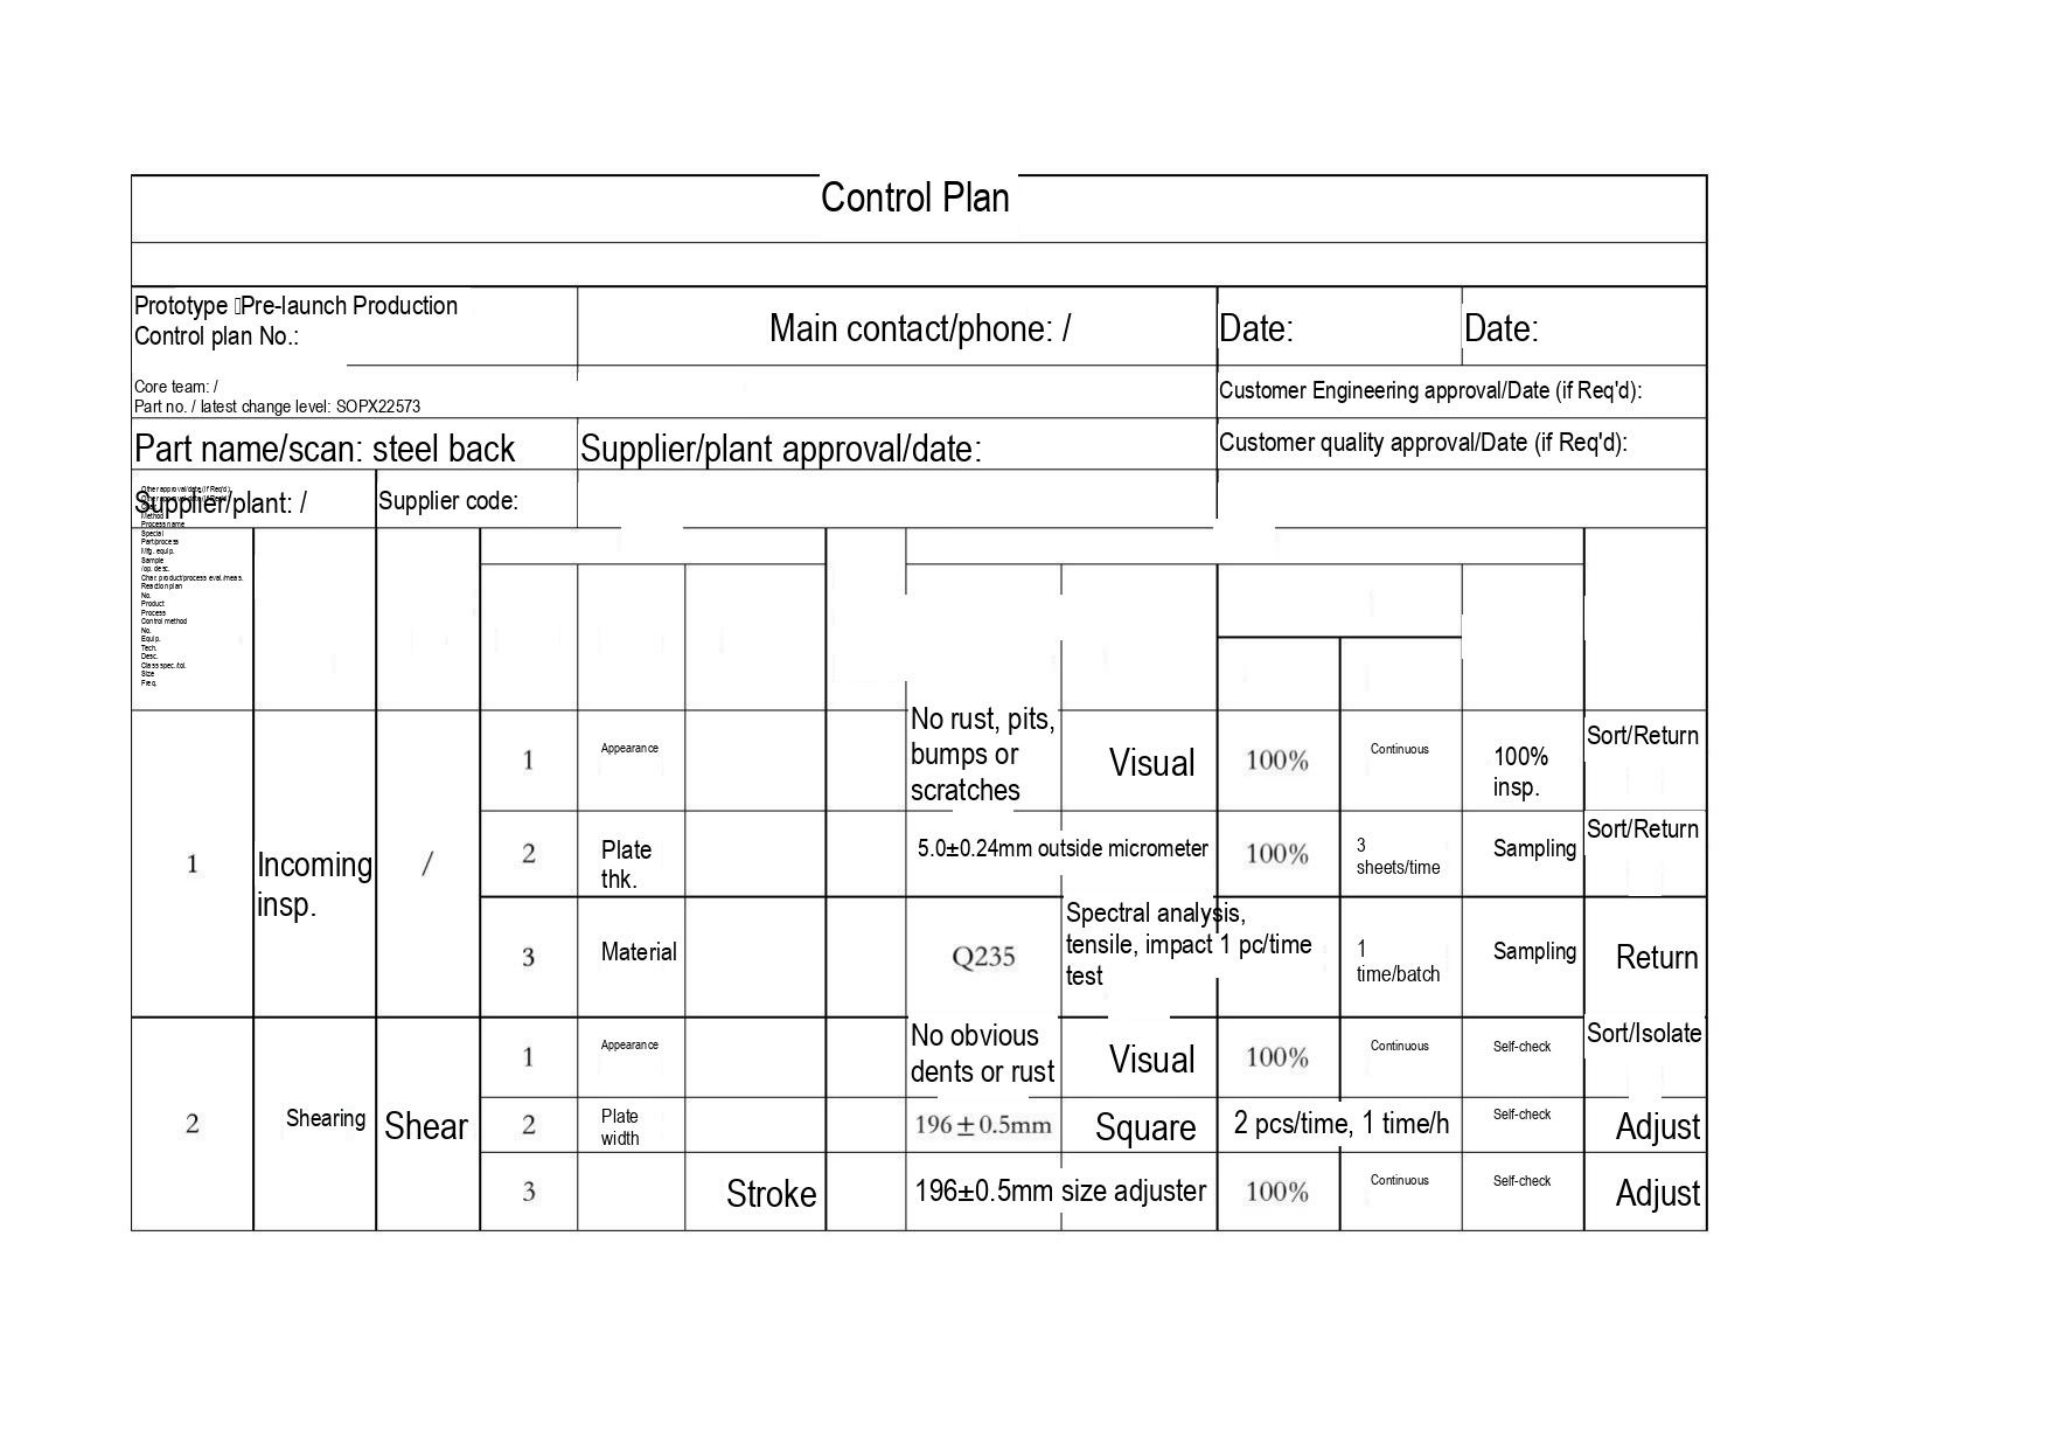Control Plan

| | | | |
|---|---|---|---|
| Prototype Pre-launch Production<br>Control plan No.: | Main contact/phone: / | Date: | Date: |
| Core team: /<br>Part no. / latest change level: SOPX22573 | | Customer Engineering approval/Date (if Req'd): | |
| Part name/scan: steel back | Supplier/plant approval/date: | Customer quality approval/Date (if Req'd): | |
| Supplier/plant: / | Supplier code: | | |

Other approval/date (If Req'd)
Method
Process name
Special
Part/process
Mfg. equip.
Sample
Op. desc.
Char. product/process eval./meas.
Reaction plan
No.
Product
Process
Control method
No.
Equip.
Tech.
Desc.
Class spec./tol.
Size
Freq.

| | | | | | | | | | | | | |
|---|---|---|---|---|---|---|---|---|---|---|---|---|
| 1 | Incoming insp. | / | 1 | Appearance | | | No rust, pits, bumps or scratches | Visual | 100% | Continuous | 100% insp. | Sort/Return |
| | | | 2 | Plate thk. | | | 5.0±0.24mm | outside micrometer | 100% | 3 sheets/time | Sampling | Sort/Return |
| | | | 3 | Material | | | Q235 | Spectral analysis, tensile, impact test | 1 pc/time | 1 time/batch | Sampling | Return |
| 2 | Shearing | Shear | 1 | Appearance | | | No obvious dents or rust | Visual | 100% | Continuous | Self-check | Sort/Isolate |
| | | | 2 | Plate width | | | 196±0.5mm | Square | 2 pcs/time, 1 time/h | | Self-check | Adjust |
| | | | 3 | | Stroke | | 196±0.5mm | size adjuster | 100% | Continuous | Self-check | Adjust |
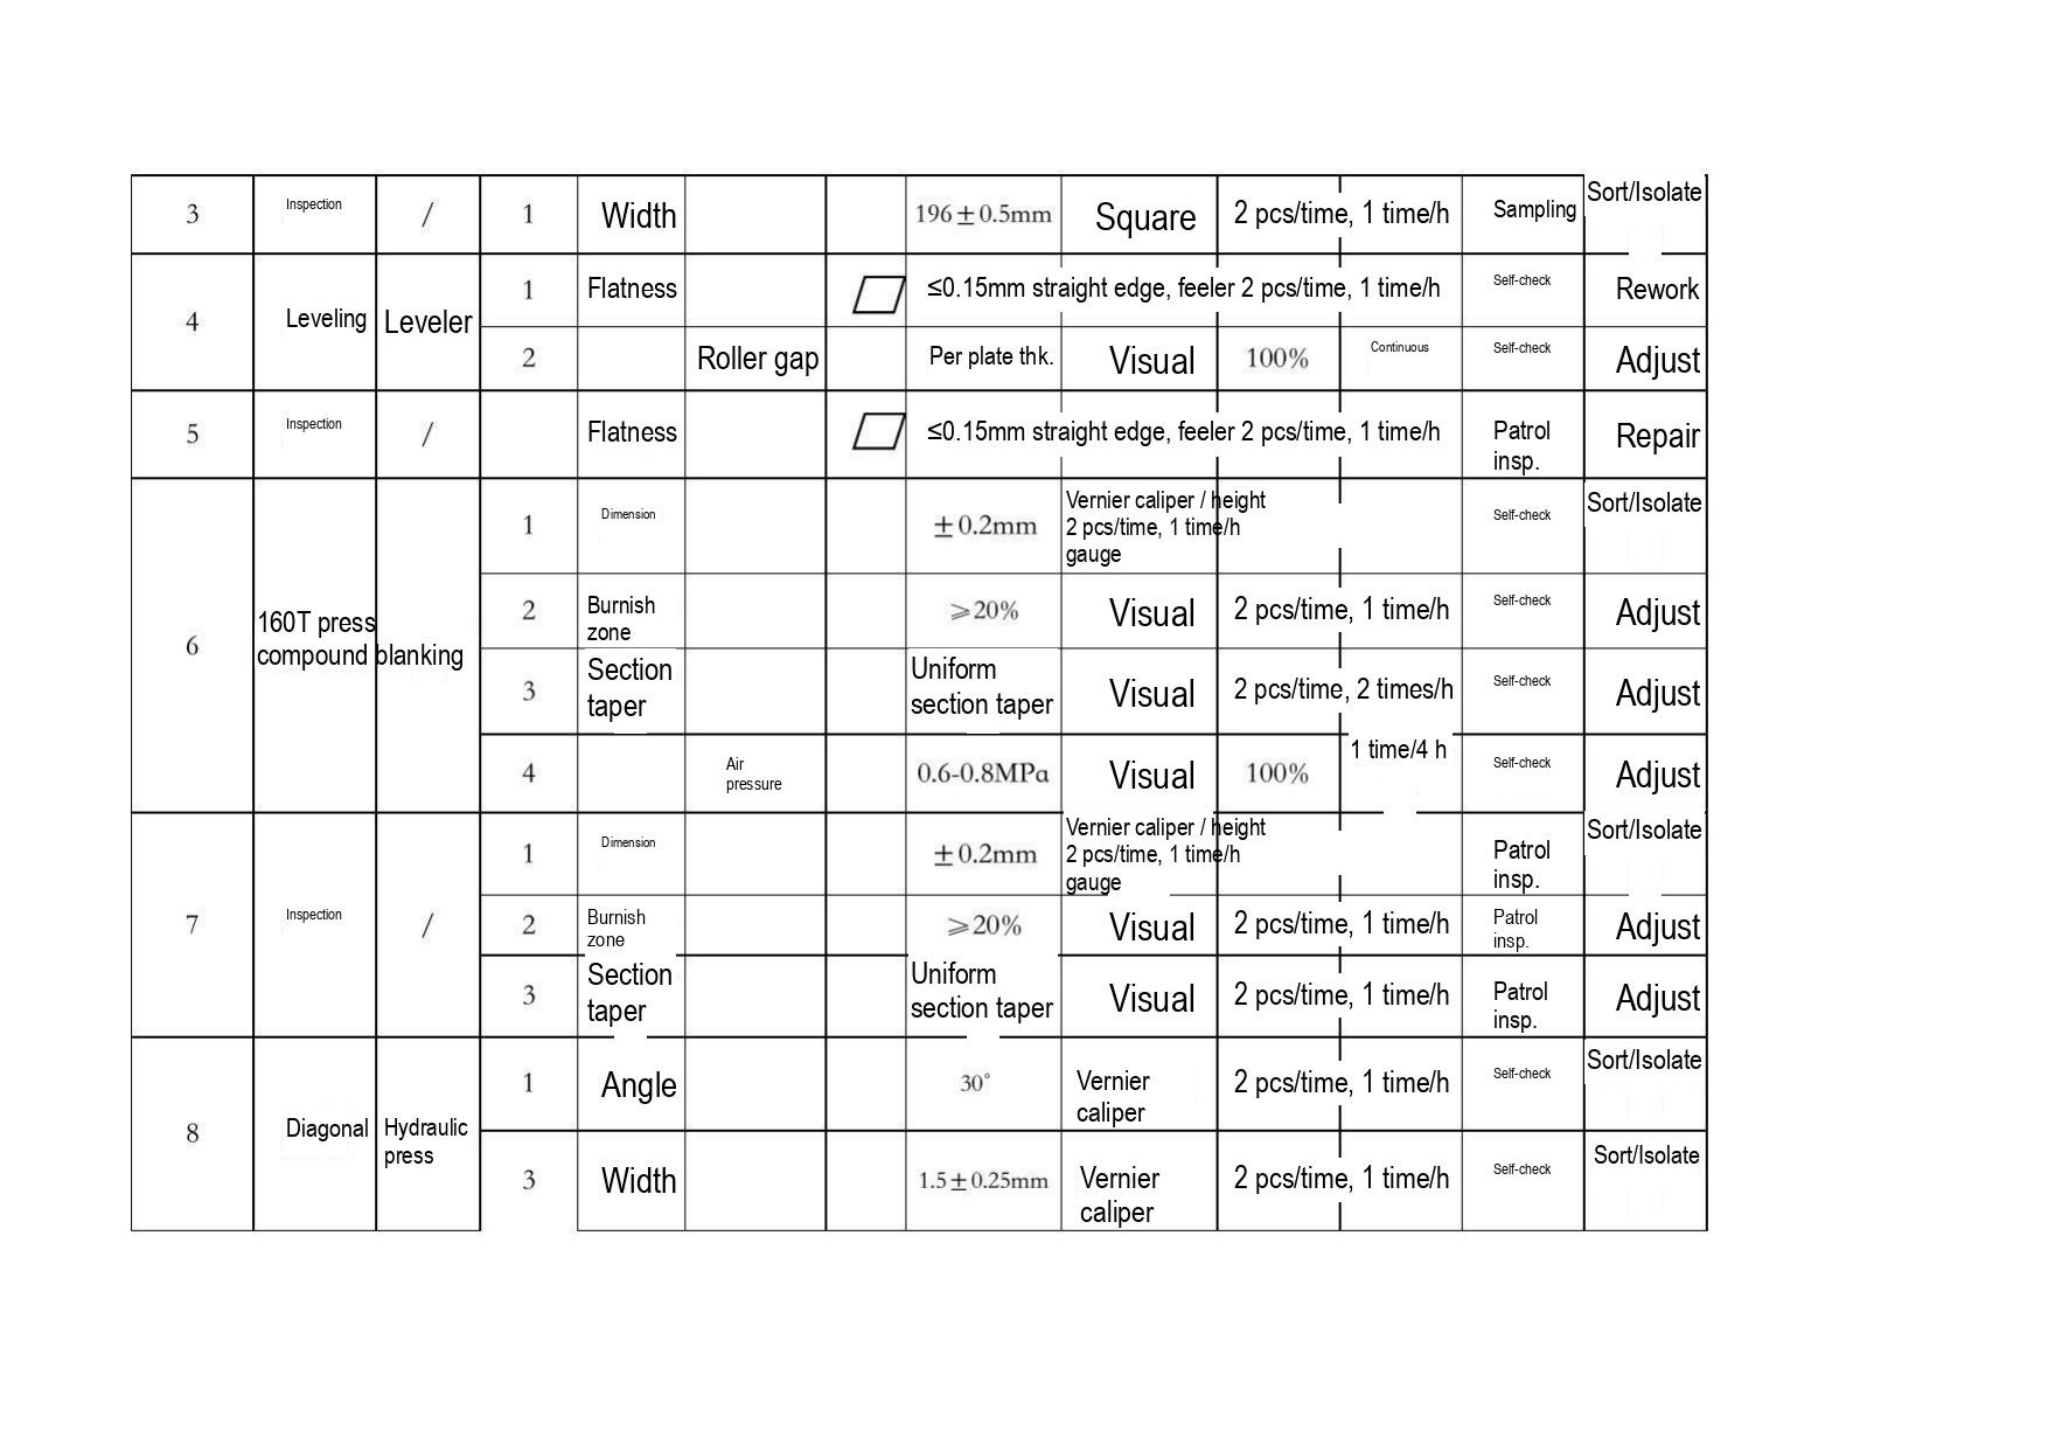|  |  |  |  |  |  |  |  |  |  |  |  |  |
|---|---|---|---|---|---|---|---|---|---|---|---|---|
| 3 | Inspection | / | 1 | Width |  |  | 196±0.5mm | Square | 2 pcs/time, 1 time/h |  | Sampling | Sort/Isolate |
| 4 | Leveling | Leveler | 1 | Flatness |  | ▱ | ≤0.15mm | straight edge, feeler | 2 pcs/time, 1 time/h |  | Self-check | Rework |
|  |  |  | 2 |  | Roller gap |  | Per plate thk. | Visual | 100% | Continuous | Self-check | Adjust |
| 5 | Inspection | / |  | Flatness |  | ▱ | ≤0.15mm | straight edge, feeler | 2 pcs/time, 1 time/h |  | Patrol insp. | Repair |
| 6 | 160T press compound blanking |  | 1 | Dimension |  |  | ±0.2mm | Vernier caliper / height gauge | 2 pcs/time, 1 time/h |  | Self-check | Sort/Isolate |
|  |  |  | 2 | Burnish zone |  |  | ≥20% | Visual | 2 pcs/time, 1 time/h |  | Self-check | Adjust |
|  |  |  | 3 | Section taper |  |  | Uniform section taper | Visual | 2 pcs/time, 2 times/h |  | Self-check | Adjust |
|  |  |  | 4 |  | Air pressure |  | 0.6-0.8MPa | Visual | 100% | 1 time/4 h | Self-check | Adjust |
| 7 | Inspection | / | 1 | Dimension |  |  | ±0.2mm | Vernier caliper / height gauge | 2 pcs/time, 1 time/h |  | Patrol insp. | Sort/Isolate |
|  |  |  | 2 | Burnish zone |  |  | ≥20% | Visual | 2 pcs/time, 1 time/h |  | Patrol insp. | Adjust |
|  |  |  | 3 | Section taper |  |  | Uniform section taper | Visual | 2 pcs/time, 1 time/h |  | Patrol insp. | Adjust |
| 8 | Diagonal | Hydraulic press | 1 | Angle |  |  | 30° | Vernier caliper | 2 pcs/time, 1 time/h |  | Self-check | Sort/Isolate |
|  |  |  | 3 | Width |  |  | 1.5±0.25mm | Vernier caliper | 2 pcs/time, 1 time/h |  | Self-check | Sort/Isolate |
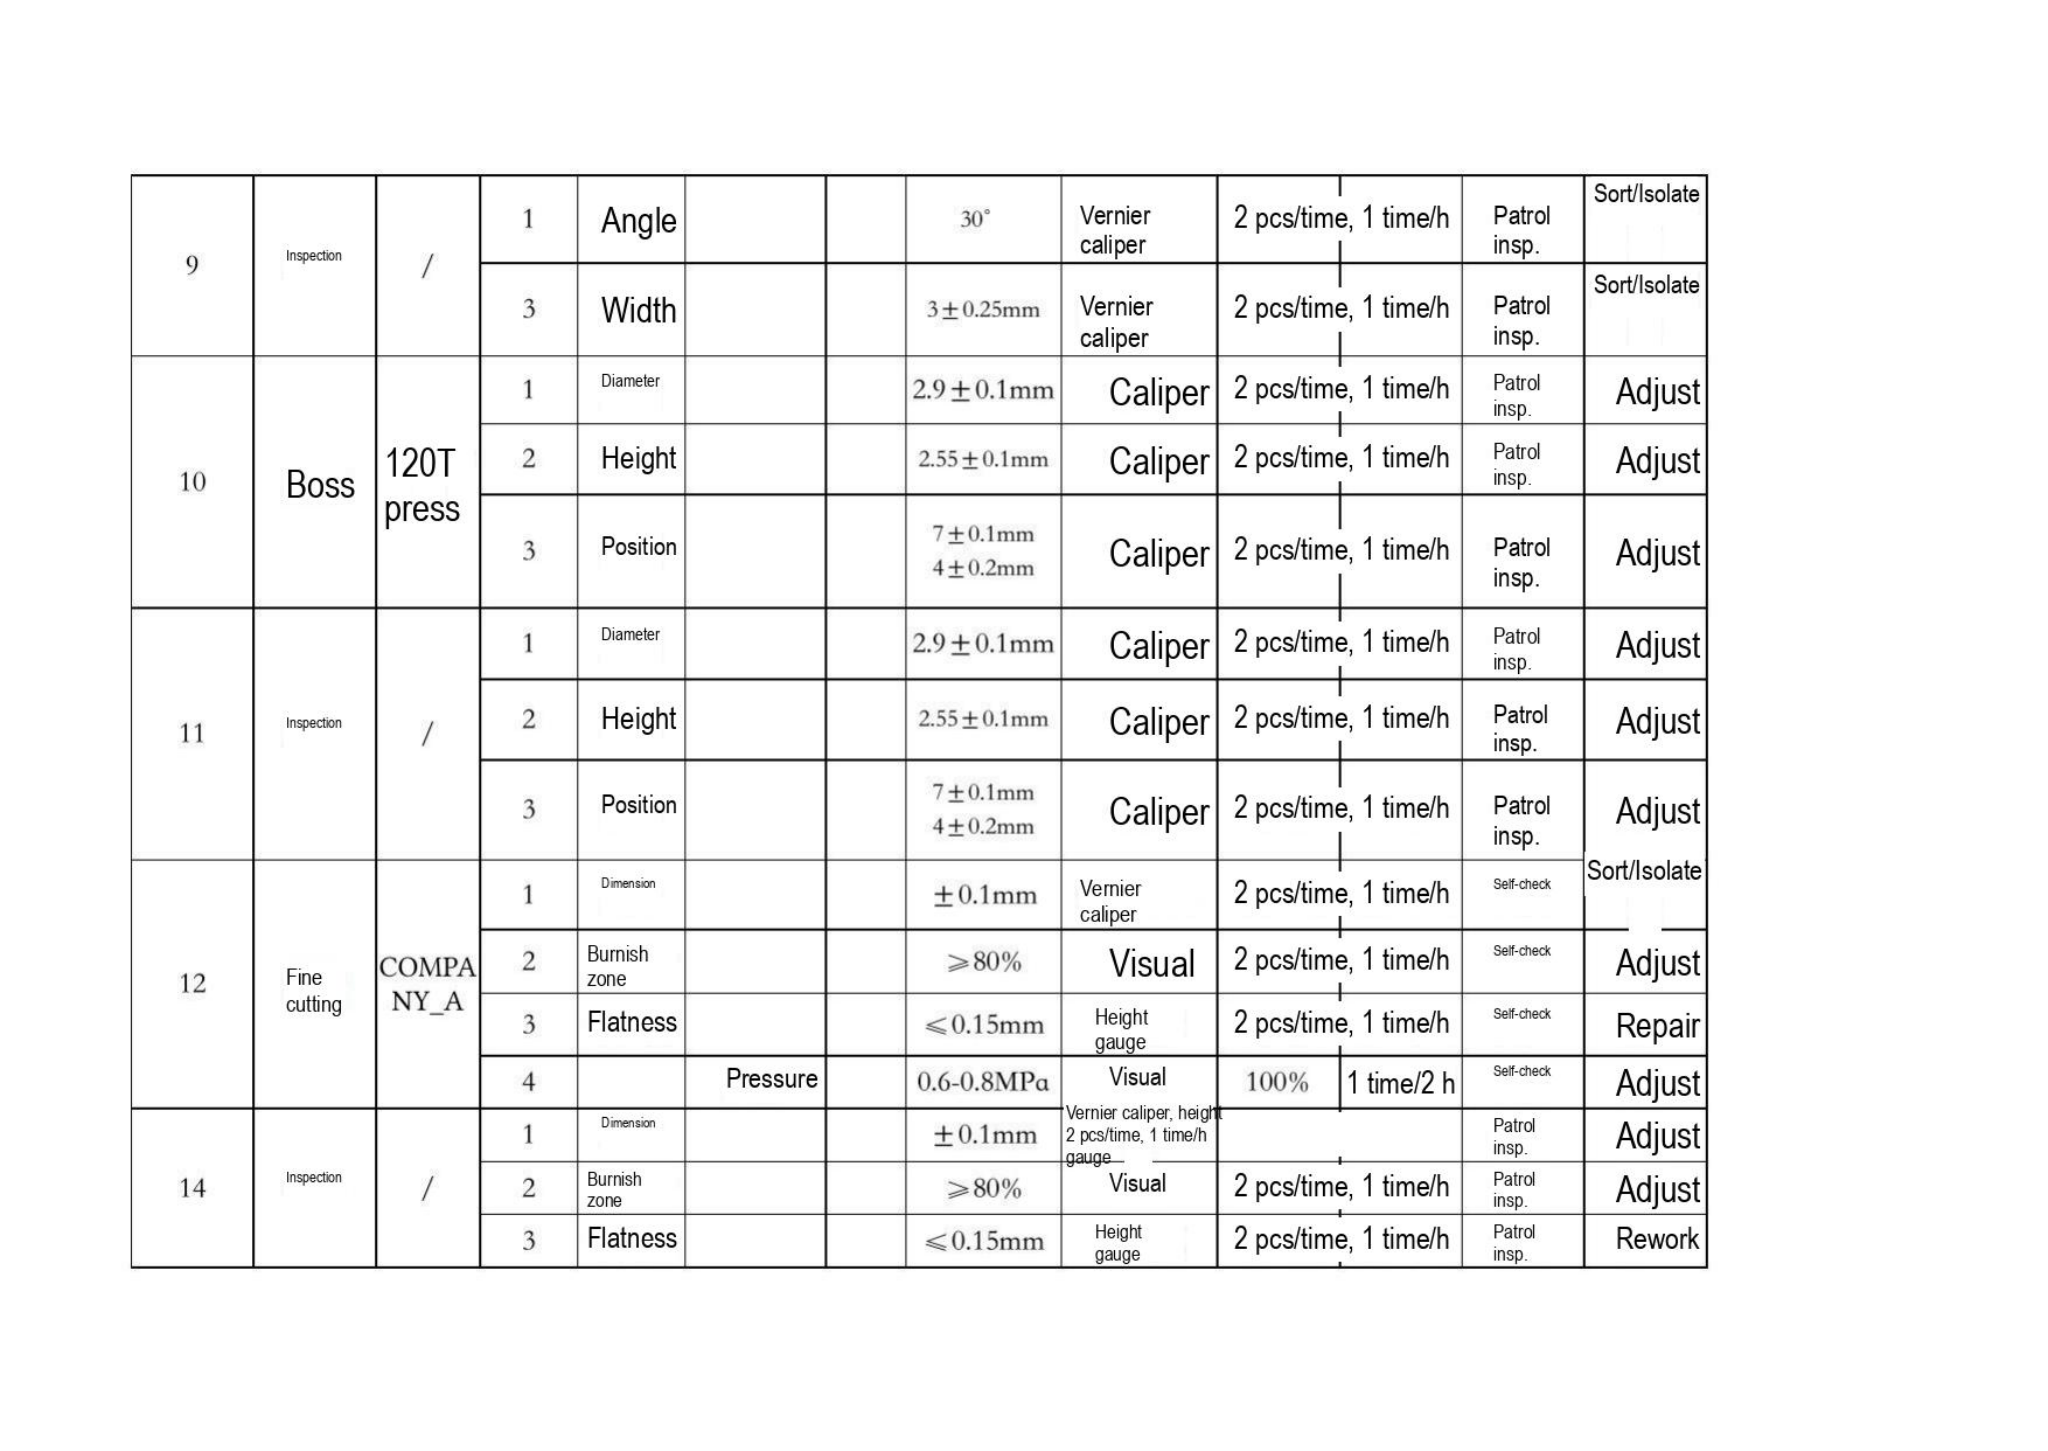|  |  |  |  |  |  |  |  |  |  |  |  |  |
|---|---|---|---|---|---|---|---|---|---|---|---|---|
| 9 | Inspection | / | 1 | Angle |  |  | 30° | Vernier caliper | 2 pcs/time, 1 time/h |  | Patrol insp. | Sort/Isolate |
|  |  |  | 3 | Width |  |  | 3±0.25mm | Vernier caliper | 2 pcs/time, 1 time/h |  | Patrol insp. | Sort/Isolate |
| 10 | Boss | 120T press | 1 | Diameter |  |  | 2.9±0.1mm | Caliper | 2 pcs/time, 1 time/h |  | Patrol insp. | Adjust |
|  |  |  | 2 | Height |  |  | 2.55±0.1mm | Caliper | 2 pcs/time, 1 time/h |  | Patrol insp. | Adjust |
|  |  |  | 3 | Position |  |  | 7±0.1mm<br>4±0.2mm | Caliper | 2 pcs/time, 1 time/h |  | Patrol insp. | Adjust |
| 11 | Inspection | / | 1 | Diameter |  |  | 2.9±0.1mm | Caliper | 2 pcs/time, 1 time/h |  | Patrol insp. | Adjust |
|  |  |  | 2 | Height |  |  | 2.55±0.1mm | Caliper | 2 pcs/time, 1 time/h |  | Patrol insp. | Adjust |
|  |  |  | 3 | Position |  |  | 7±0.1mm<br>4±0.2mm | Caliper | 2 pcs/time, 1 time/h |  | Patrol insp. | Adjust |
| 12 | Fine cutting | COMPANY_A | 1 | Dimension |  |  | ±0.1mm | Vernier caliper | 2 pcs/time, 1 time/h |  | Self-check | Sort/Isolate |
|  |  |  | 2 | Burnish zone |  |  | ≥80% | Visual | 2 pcs/time, 1 time/h |  | Self-check | Adjust |
|  |  |  | 3 | Flatness |  |  | ≤0.15mm | Height gauge | 2 pcs/time, 1 time/h |  | Self-check | Repair |
|  |  |  | 4 |  | Pressure |  | 0.6-0.8MPa | Visual | 100% | 1 time/2 h | Self-check | Adjust |
| 14 | Inspection | / | 1 | Dimension |  |  | ±0.1mm | Vernier caliper, height gauge | 2 pcs/time, 1 time/h |  | Patrol insp. | Adjust |
|  |  |  | 2 | Burnish zone |  |  | ≥80% | Visual | 2 pcs/time, 1 time/h |  | Patrol insp. | Adjust |
|  |  |  | 3 | Flatness |  |  | ≤0.15mm | Height gauge | 2 pcs/time, 1 time/h |  | Patrol insp. | Rework |
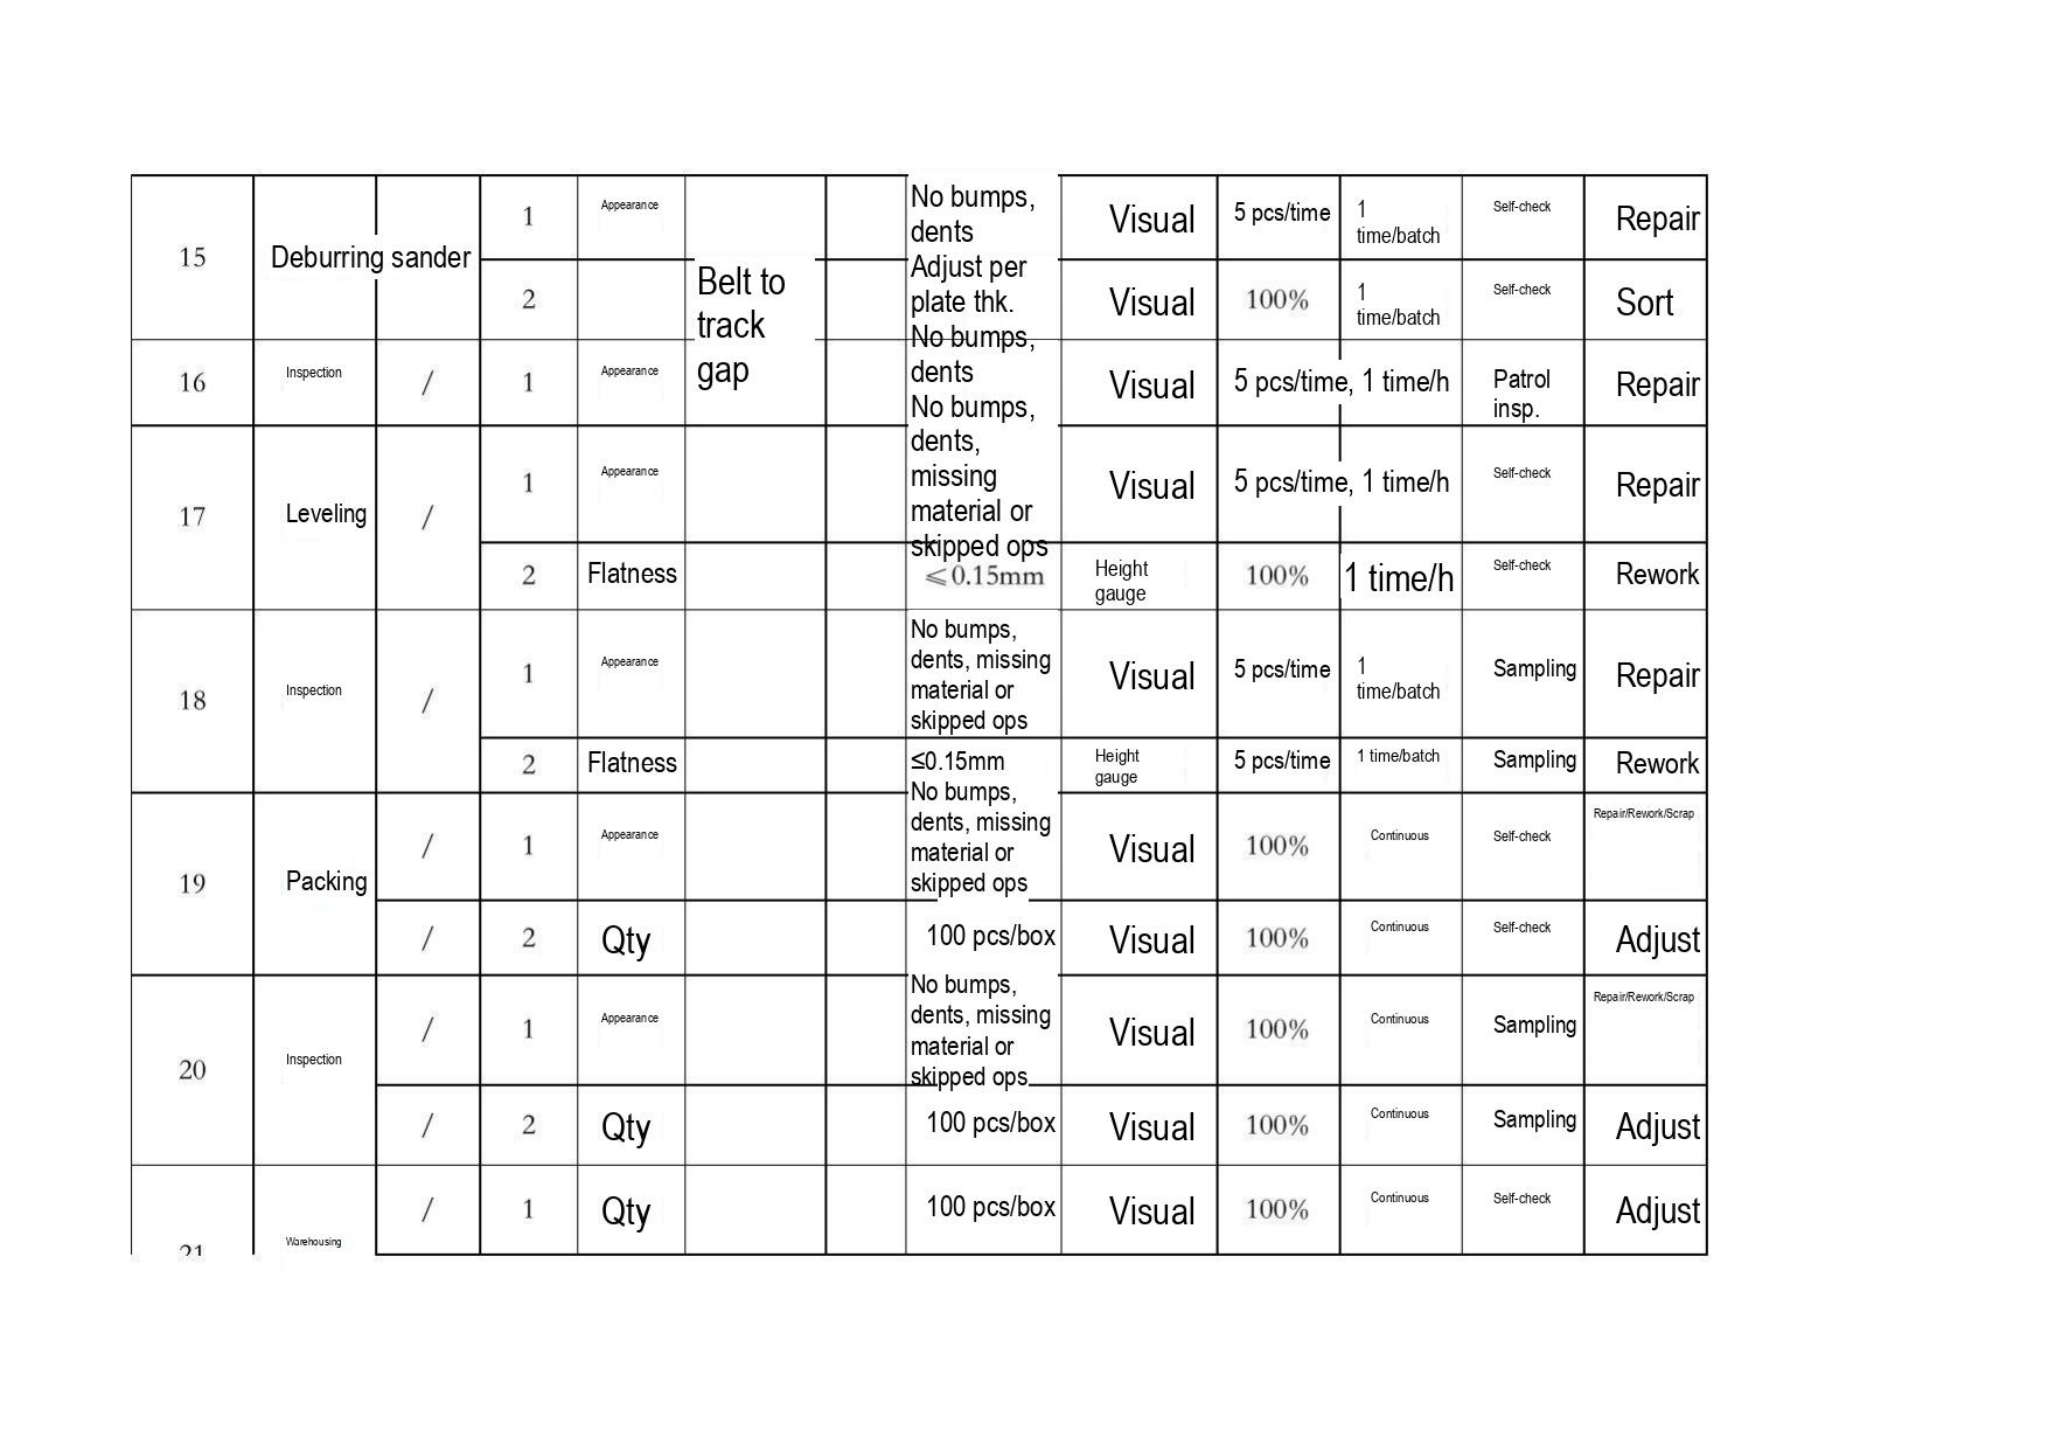| | | | | | | | | | | | | |
|---|---|---|---|---|---|---|---|---|---|---|---|---|
| 15 | Deburring sander | | 1 | Appearance | | | No bumps, dents | Visual | 5 pcs/time | 1 time/batch | Self-check | Repair |
| | | | 2 | | Belt to track gap | | Adjust per plate thk. | Visual | 100% | 1 time/batch | Self-check | Sort |
| 16 | Inspection | / | 1 | Appearance | | | No bumps, dents | Visual | 5 pcs/time, 1 time/h | | Patrol insp. | Repair |
| 17 | Leveling | / | 1 | Appearance | | | No bumps, dents, missing material or skipped ops | Visual | 5 pcs/time, 1 time/h | | Self-check | Repair |
| | | | 2 | Flatness | | | ≤0.15mm | Height gauge | 100% | 1 time/h | Self-check | Rework |
| 18 | Inspection | / | 1 | Appearance | | | No bumps, dents, missing material or skipped ops | Visual | 5 pcs/time | 1 time/batch | Sampling | Repair |
| | | | 2 | Flatness | | | ≤0.15mm | Height gauge | 5 pcs/time | 1 time/batch | Sampling | Rework |
| 19 | Packing | / | 1 | Appearance | | | No bumps, dents, missing material or skipped ops | Visual | 100% | Continuous | Self-check | Repair/Rework/Scrap |
| | | / | 2 | Qty | | | 100 pcs/box | Visual | 100% | Continuous | Self-check | Adjust |
| 20 | Inspection | / | 1 | Appearance | | | No bumps, dents, missing material or skipped ops | Visual | 100% | Continuous | Sampling | Repair/Rework/Scrap |
| | | / | 2 | Qty | | | 100 pcs/box | Visual | 100% | Continuous | Sampling | Adjust |
| 21 | Warehousing | / | 1 | Qty | | | 100 pcs/box | Visual | 100% | Continuous | Self-check | Adjust |
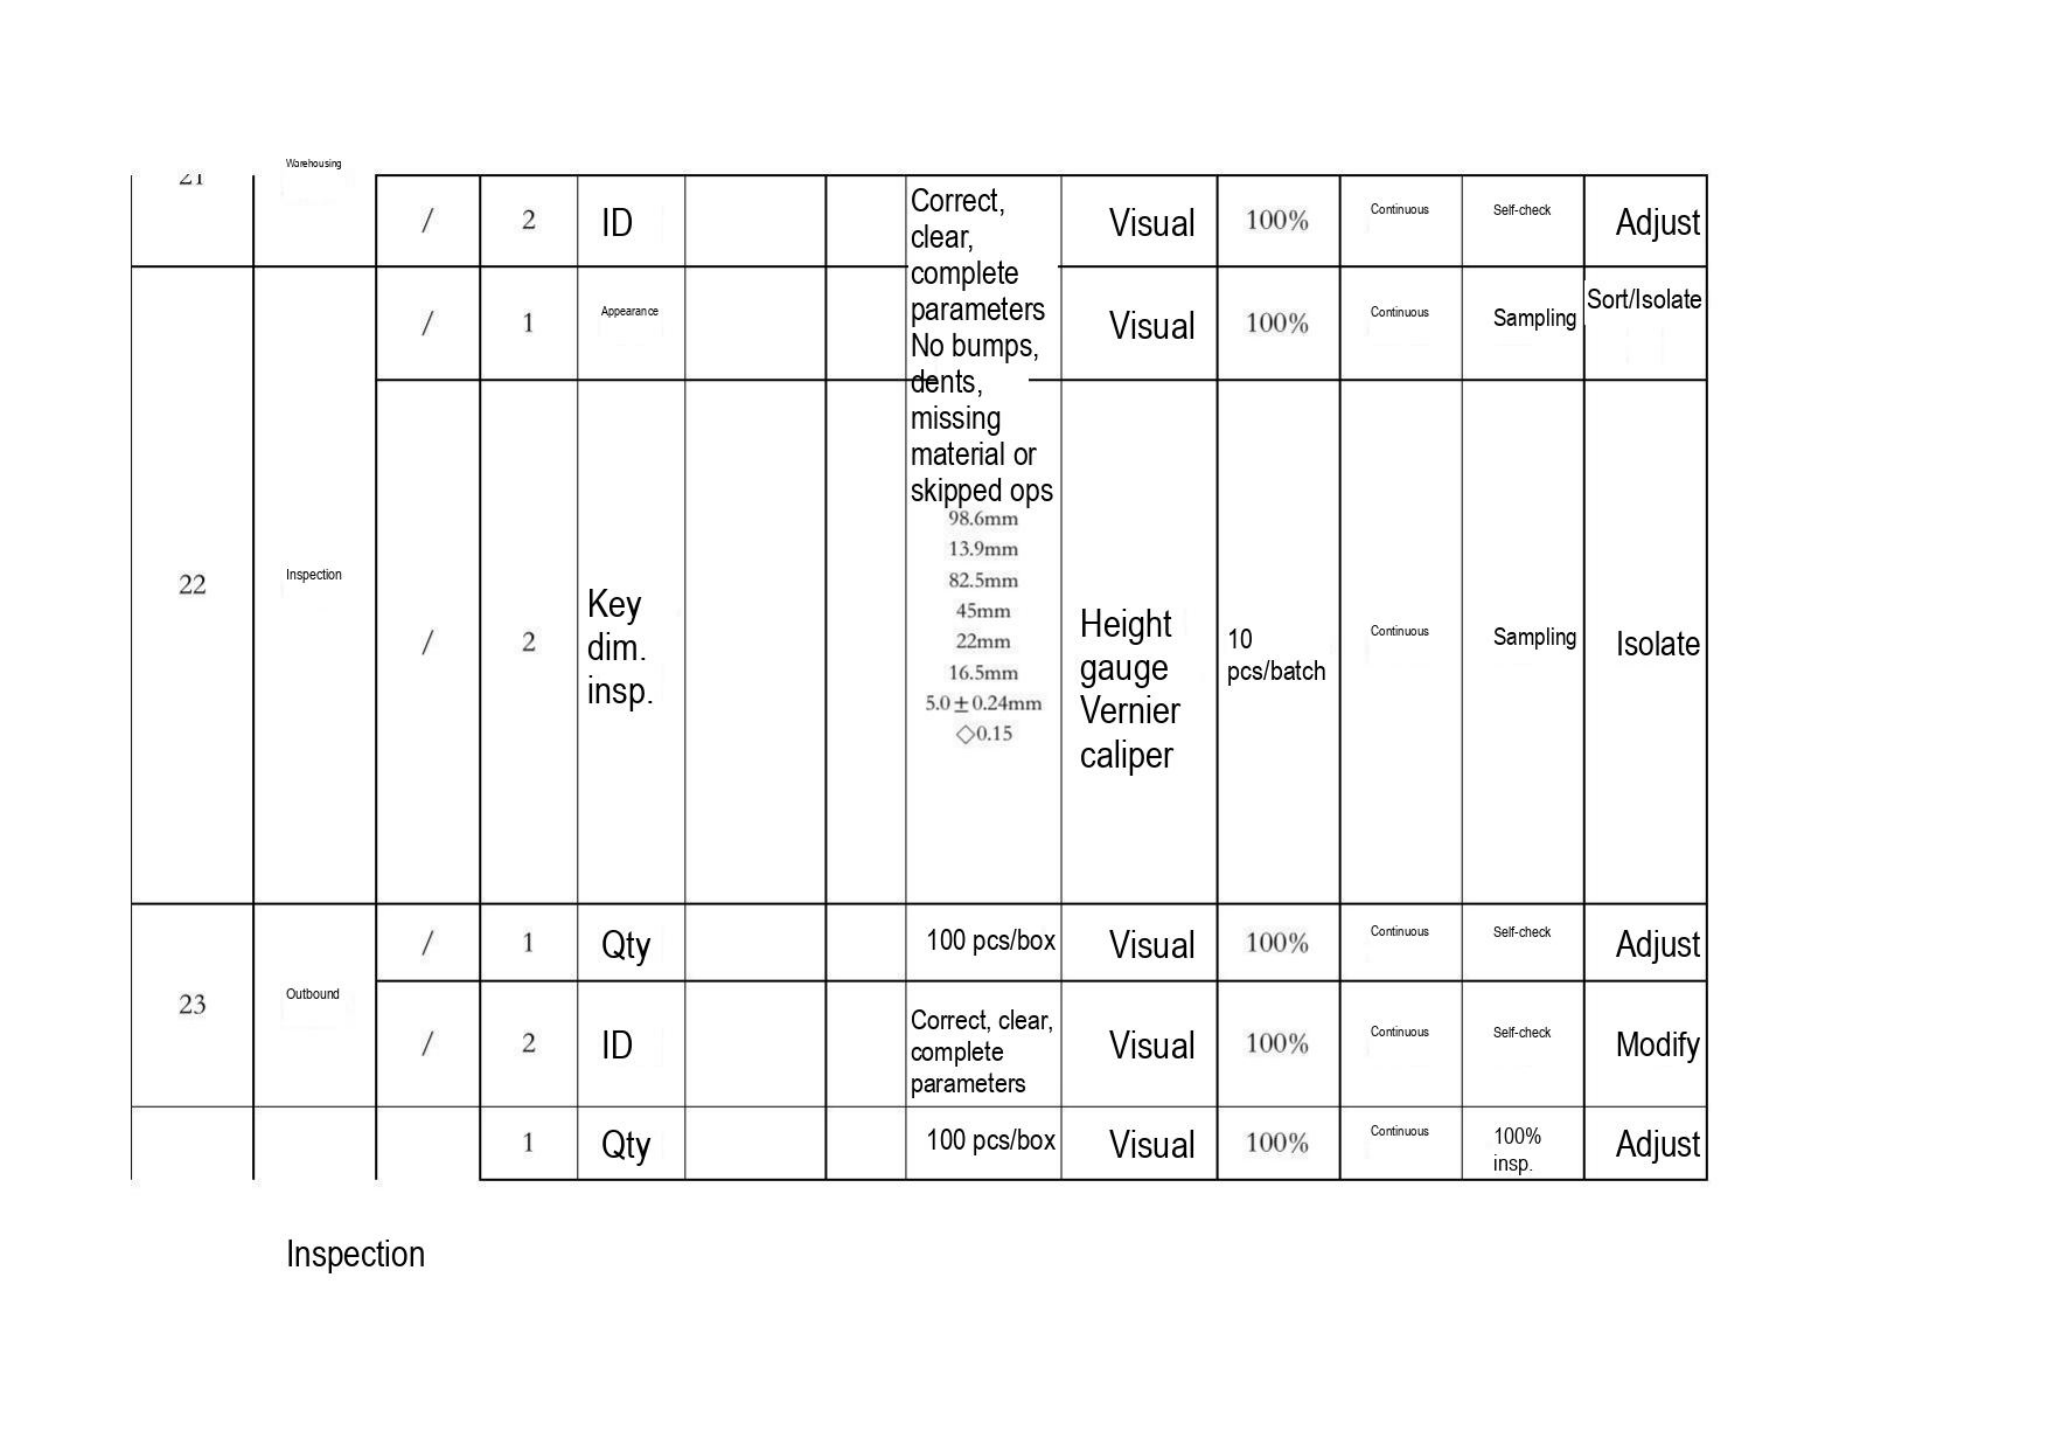| 21 | Warehousing | | | | | | | | | | | |
|---|---|---|---|---|---|---|---|---|---|---|---|---|
| | | / | 2 | ID | | | Correct, clear, complete parameters | Visual | 100% | Continuous | Self-check | Adjust |
| 22 | Inspection | / | 1 | Appearance | | | No bumps, dents, missing material or skipped ops | Visual | 100% | Continuous | Sampling | Sort/Isolate |
| | | / | 2 | Key dim. insp. | | | 98.6mm<br>13.9mm<br>82.5mm<br>45mm<br>22mm<br>16.5mm<br>5.0±0.24mm<br>◇0.15 | Height gauge Vernier caliper | 10 pcs/batch | Continuous | Sampling | Isolate |
| 23 | Outbound | / | 1 | Qty | | | 100 pcs/box | Visual | 100% | Continuous | Self-check | Adjust |
| | | / | 2 | ID | | | Correct, clear, complete parameters | Visual | 100% | Continuous | Self-check | Modify |
| | | | 1 | Qty | | | 100 pcs/box | Visual | 100% | Continuous | 100% insp. | Adjust |

Inspection
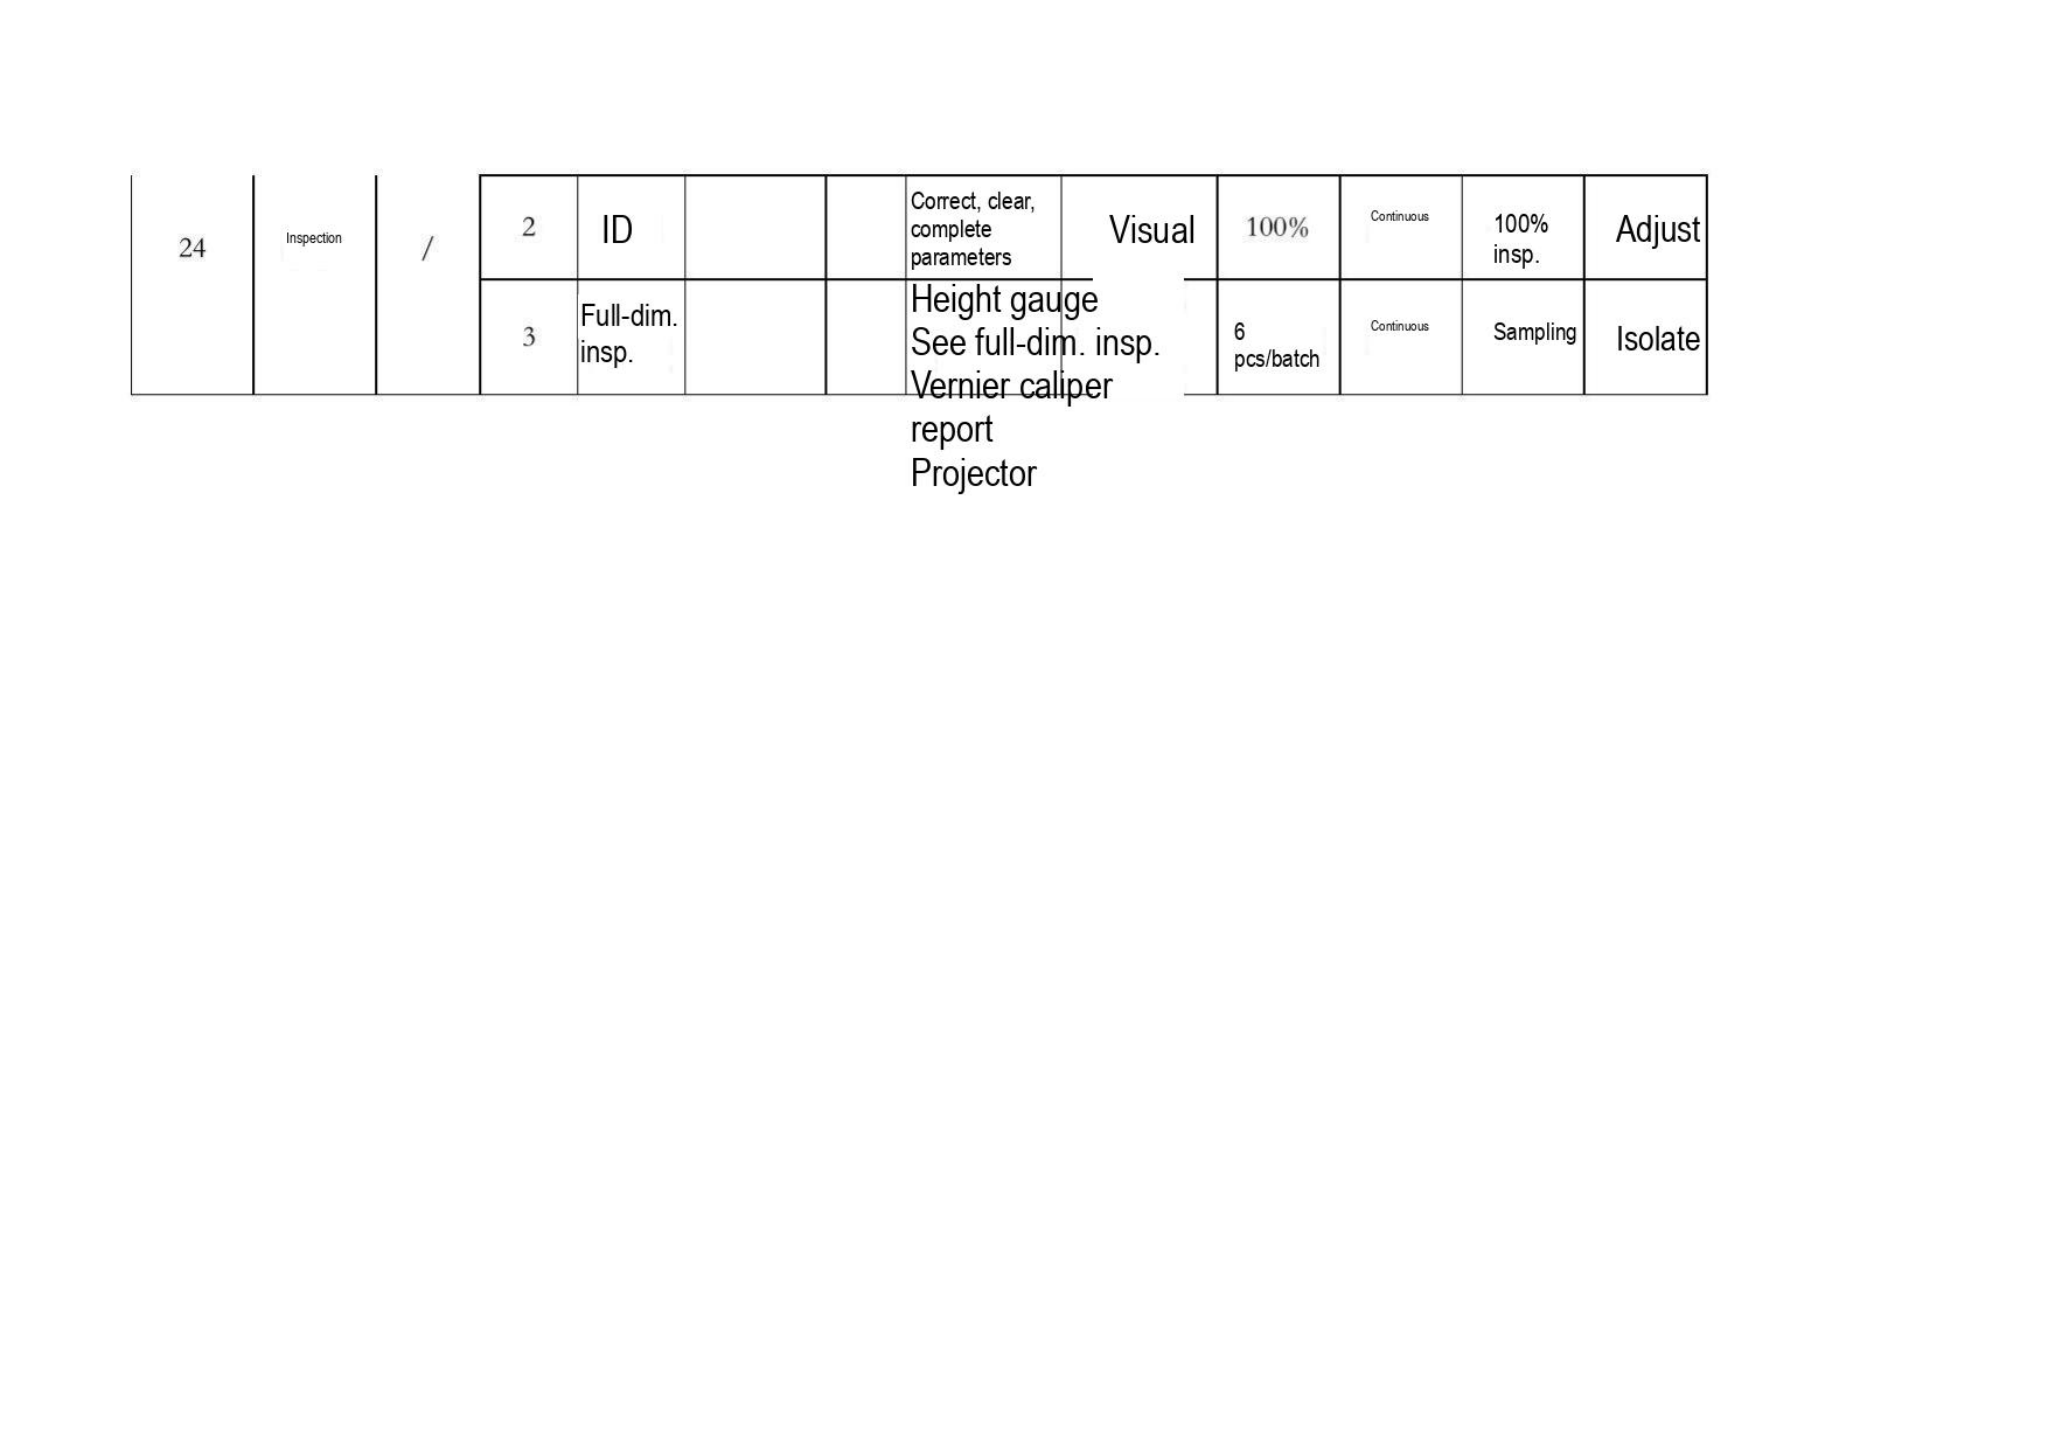|  |  |  |  |  |  |  |  |  |  |  |  |  |
|---|---|---|---|---|---|---|---|---|---|---|---|---|
| 24 | Inspection | / | 2 | ID |  |  | Correct, clear, complete parameters | Visual | 100% | Continuous | 100% insp. | Adjust |
|  |  |  | 3 | Full-dim. insp. |  |  | Height gauge<br>See full-dim. insp.<br>Vernier caliper<br>report<br>Projector |  | 6 pcs/batch | Continuous | Sampling | Isolate |